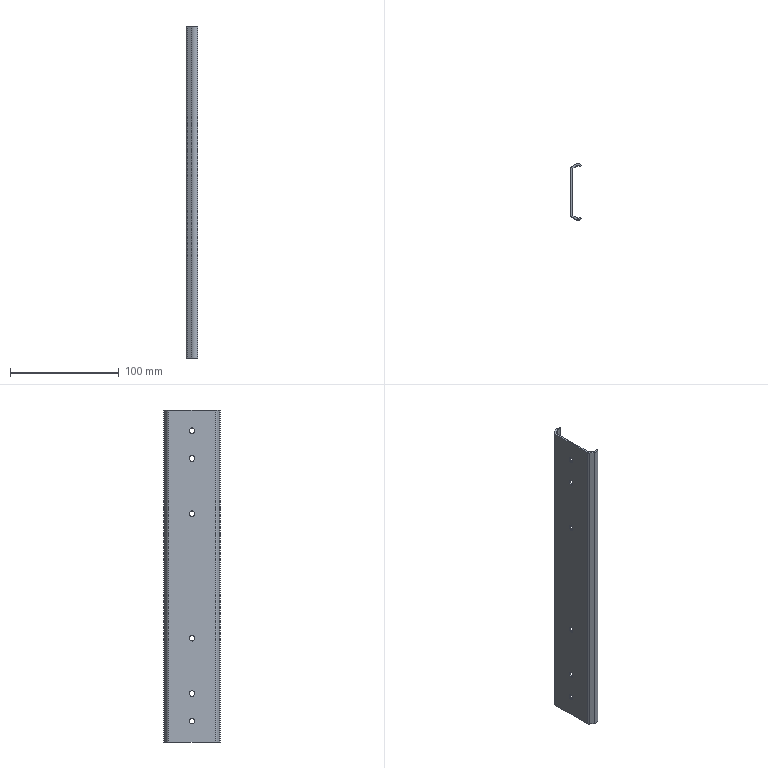Part | SolidWorks | features BaseBody 1 | 1 solid | 48 faces | box 10.262 x 51.5 x 305 mm | volume 30693 mm3 | cylinder 26 | plane 22 | commonest cylinder face diameters 4.5 x18 2.853 x2 3.795 x2 5.56 x2 8.66 x2